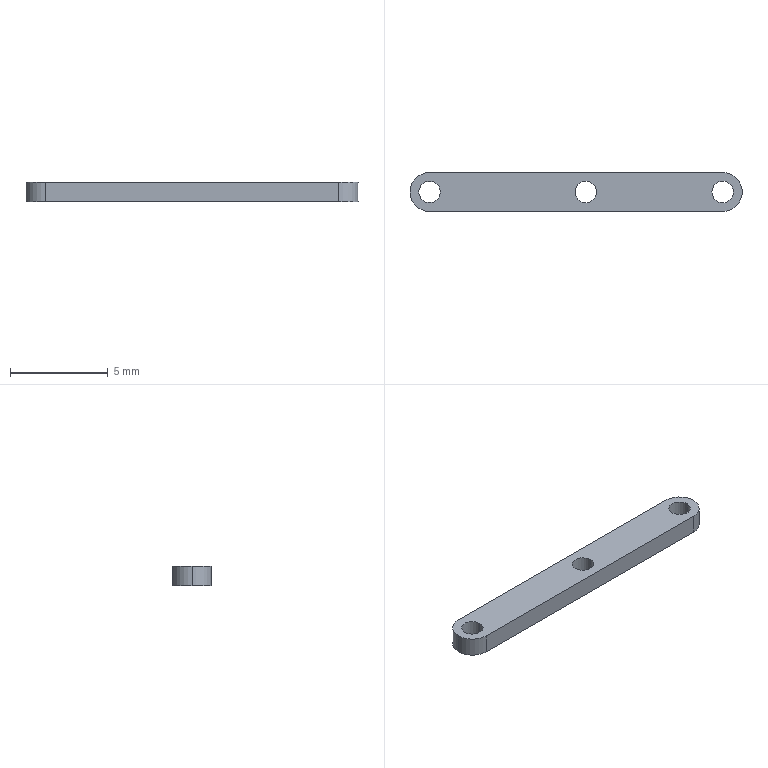Part | SolidWorks | features Extrusion 1, ICE 1 | 1 solid | 13 faces | box 17 x 2 x 1 mm | volume 30.291 mm3 | cylinder 9 | plane 4 | commonest cylinder face diameters 1.1 x6 2 x3
STEP:
#1=CARTESIAN_POINT('',(-0.05,0.,0.5));
#2=VERTEX_POINT('',#1);
#3=CARTESIAN_POINT('',(1.05,0.,0.5));
#4=VERTEX_POINT('',#3);
#5=CARTESIAN_POINT('',(0.5,0.,0.5));
#6=DIRECTION('',(0.,0.,1.));
#7=DIRECTION('',(1.,0.,0.));
#8=AXIS2_PLACEMENT_3D('',#5,#6,#7);
#9=CIRCLE('',#8,0.55);
#10=EDGE_CURVE('',#2,#4,#9,.T.);
#11=ORIENTED_EDGE('',*,*,#10,.T.);
#12=CARTESIAN_POINT('',(1.05,0.,-0.5));
#13=VERTEX_POINT('',#12);
#14=CARTESIAN_POINT('',(1.05,0.,0.5));
#15=DIRECTION('',(0.,0.,-1.));
#16=VECTOR('',#15,1000.);
#17=LINE('',#14,#16);
#18=EDGE_CURVE('',#4,#13,#17,.T.);
#19=ORIENTED_EDGE('',*,*,#18,.T.);
#20=CARTESIAN_POINT('',(-0.05,0.,-0.5));
#21=VERTEX_POINT('',#20);
#22=CARTESIAN_POINT('',(0.5,0.,-0.5));
#23=DIRECTION('',(0.,0.,1.));
#24=DIRECTION('',(1.,0.,0.));
#25=AXIS2_PLACEMENT_3D('',#22,#23,#24);
#26=CIRCLE('',#25,0.55);
#27=EDGE_CURVE('',#21,#13,#26,.T.);
#28=ORIENTED_EDGE('',*,*,#27,.F.);
#29=CARTESIAN_POINT('',(-0.05,0.,0.5));
#30=DIRECTION('',(0.,0.,-1.));
#31=VECTOR('',#30,1000.);
#32=LINE('',#29,#31);
#33=EDGE_CURVE('',#2,#21,#32,.T.);
#34=ORIENTED_EDGE('',*,*,#33,.F.);
#35=EDGE_LOOP('',(#11,#19,#28,#34));
#36=FACE_OUTER_BOUND('',#35,.T.);
#37=CARTESIAN_POINT('',(0.5,0.,0.5));
#38=DIRECTION('',(0.,0.,-1.));
#39=DIRECTION('',(-1.,0.,0.));
#40=AXIS2_PLACEMENT_3D('',#37,#38,#39);
#41=CYLINDRICAL_SURFACE('',#40,0.55);
#42=ADVANCED_FACE('',(#36),#41,.F.);
#43=CARTESIAN_POINT('',(6.95,0.,0.5));
#44=VERTEX_POINT('',#43);
#45=CARTESIAN_POINT('',(8.05,0.,0.5));
#46=VERTEX_POINT('',#45);
#47=CARTESIAN_POINT('',(7.5,0.,0.5));
#48=DIRECTION('',(0.,0.,1.));
#49=DIRECTION('',(1.,0.,0.));
#50=AXIS2_PLACEMENT_3D('',#47,#48,#49);
#51=CIRCLE('',#50,0.55);
#52=EDGE_CURVE('',#44,#46,#51,.T.);
#53=ORIENTED_EDGE('',*,*,#52,.T.);
#54=CARTESIAN_POINT('',(8.05,0.,-0.5));
#55=VERTEX_POINT('',#54);
#56=CARTESIAN_POINT('',(8.05,0.,0.5));
#57=DIRECTION('',(0.,0.,-1.));
#58=VECTOR('',#57,1000.);
#59=LINE('',#56,#58);
#60=EDGE_CURVE('',#46,#55,#59,.T.);
#61=ORIENTED_EDGE('',*,*,#60,.T.);
#62=CARTESIAN_POINT('',(6.95,0.,-0.5));
#63=VERTEX_POINT('',#62);
#64=CARTESIAN_POINT('',(7.5,0.,-0.5));
#65=DIRECTION('',(0.,0.,1.));
#66=DIRECTION('',(1.,0.,0.));
#67=AXIS2_PLACEMENT_3D('',#64,#65,#66);
#68=CIRCLE('',#67,0.55);
#69=EDGE_CURVE('',#63,#55,#68,.T.);
#70=ORIENTED_EDGE('',*,*,#69,.F.);
#71=CARTESIAN_POINT('',(6.95,0.,0.5));
#72=DIRECTION('',(0.,0.,-1.));
#73=VECTOR('',#72,1000.);
#74=LINE('',#71,#73);
#75=EDGE_CURVE('',#44,#63,#74,.T.);
#76=ORIENTED_EDGE('',*,*,#75,.F.);
#77=EDGE_LOOP('',(#53,#61,#70,#76));
#78=FACE_OUTER_BOUND('',#77,.T.);
#79=CARTESIAN_POINT('',(7.5,0.,0.5));
#80=DIRECTION('',(0.,0.,-1.));
#81=DIRECTION('',(-1.,0.,0.));
#82=AXIS2_PLACEMENT_3D('',#79,#80,#81);
#83=CYLINDRICAL_SURFACE('',#82,0.55);
#84=ADVANCED_FACE('',(#78),#83,.F.);
#85=CARTESIAN_POINT('',(-8.05,0.,0.5));
#86=VERTEX_POINT('',#85);
#87=CARTESIAN_POINT('',(-6.95,0.,0.5));
#88=VERTEX_POINT('',#87);
#89=CARTESIAN_POINT('',(-7.5,0.,0.5));
#90=DIRECTION('',(0.,0.,1.));
#91=DIRECTION('',(1.,0.,0.));
#92=AXIS2_PLACEMENT_3D('',#89,#90,#91);
#93=CIRCLE('',#92,0.55);
#94=EDGE_CURVE('',#86,#88,#93,.T.);
#95=ORIENTED_EDGE('',*,*,#94,.T.);
#96=CARTESIAN_POINT('',(-6.95,0.,-0.5));
#97=VERTEX_POINT('',#96);
#98=CARTESIAN_POINT('',(-6.95,0.,0.5));
#99=DIRECTION('',(0.,0.,-1.));
#100=VECTOR('',#99,1000.);
#101=LINE('',#98,#100);
#102=EDGE_CURVE('',#88,#97,#101,.T.);
#103=ORIENTED_EDGE('',*,*,#102,.T.);
#104=CARTESIAN_POINT('',(-8.05,0.,-0.5));
#105=VERTEX_POINT('',#104);
#106=CARTESIAN_POINT('',(-7.5,0.,-0.5));
#107=DIRECTION('',(0.,0.,1.));
#108=DIRECTION('',(1.,0.,0.));
#109=AXIS2_PLACEMENT_3D('',#106,#107,#108);
#110=CIRCLE('',#109,0.55);
#111=EDGE_CURVE('',#105,#97,#110,.T.);
#112=ORIENTED_EDGE('',*,*,#111,.F.);
#113=CARTESIAN_POINT('',(-8.05,0.,0.5));
#114=DIRECTION('',(0.,0.,-1.));
#115=VECTOR('',#114,1000.);
#116=LINE('',#113,#115);
#117=EDGE_CURVE('',#86,#105,#116,.T.);
#118=ORIENTED_EDGE('',*,*,#117,.F.);
#119=EDGE_LOOP('',(#95,#103,#112,#118));
#120=FACE_OUTER_BOUND('',#119,.T.);
#121=CARTESIAN_POINT('',(-7.5,0.,0.5));
#122=DIRECTION('',(0.,0.,-1.));
#123=DIRECTION('',(-1.,0.,0.));
#124=AXIS2_PLACEMENT_3D('',#121,#122,#123);
#125=CYLINDRICAL_SURFACE('',#124,0.55);
#126=ADVANCED_FACE('',(#120),#125,.F.);
#127=CARTESIAN_POINT('',(-8.5,0.,0.5));
#128=VERTEX_POINT('',#127);
#129=CARTESIAN_POINT('',(-7.5,-1.,0.5));
#130=VERTEX_POINT('',#129);
#131=CARTESIAN_POINT('',(-7.5,0.,0.5));
#132=DIRECTION('',(0.,0.,1.));
#133=DIRECTION('',(1.,0.,0.));
#134=AXIS2_PLACEMENT_3D('',#131,#132,#133);
#135=CIRCLE('',#134,1.);
#136=EDGE_CURVE('',#128,#130,#135,.T.);
#137=ORIENTED_EDGE('',*,*,#136,.F.);
#138=CARTESIAN_POINT('',(-8.5,0.,-0.5));
#139=VERTEX_POINT('',#138);
#140=CARTESIAN_POINT('',(-8.5,0.,0.5));
#141=DIRECTION('',(0.,0.,-1.));
#142=VECTOR('',#141,1000.);
#143=LINE('',#140,#142);
#144=EDGE_CURVE('',#128,#139,#143,.T.);
#145=ORIENTED_EDGE('',*,*,#144,.T.);
#146=CARTESIAN_POINT('',(-7.5,-1.,-0.5));
#147=VERTEX_POINT('',#146);
#148=CARTESIAN_POINT('',(-7.5,0.,-0.5));
#149=DIRECTION('',(0.,0.,1.));
#150=DIRECTION('',(1.,0.,0.));
#151=AXIS2_PLACEMENT_3D('',#148,#149,#150);
#152=CIRCLE('',#151,1.);
#153=EDGE_CURVE('',#139,#147,#152,.T.);
#154=ORIENTED_EDGE('',*,*,#153,.T.);
#155=CARTESIAN_POINT('',(-7.5,-1.,0.5));
#156=DIRECTION('',(0.,0.,-1.));
#157=VECTOR('',#156,1000.);
#158=LINE('',#155,#157);
#159=EDGE_CURVE('',#130,#147,#158,.T.);
#160=ORIENTED_EDGE('',*,*,#159,.F.);
#161=EDGE_LOOP('',(#137,#145,#154,#160));
#162=FACE_OUTER_BOUND('',#161,.T.);
#163=CARTESIAN_POINT('',(-7.5,0.,0.5));
#164=DIRECTION('',(0.,0.,-1.));
#165=DIRECTION('',(-1.,0.,0.));
#166=AXIS2_PLACEMENT_3D('',#163,#164,#165);
#167=CYLINDRICAL_SURFACE('',#166,1.);
#168=ADVANCED_FACE('',(#162),#167,.T.);
#169=ORIENTED_EDGE('',*,*,#52,.F.);
#170=CARTESIAN_POINT('',(7.5,0.,0.5));
#171=DIRECTION('',(0.,0.,1.));
#172=DIRECTION('',(1.,0.,0.));
#173=AXIS2_PLACEMENT_3D('',#170,#171,#172);
#174=CIRCLE('',#173,0.55);
#175=EDGE_CURVE('',#46,#44,#174,.T.);
#176=ORIENTED_EDGE('',*,*,#175,.F.);
#177=EDGE_LOOP('',(#169,#176));
#178=FACE_BOUND('',#177,.T.);
#179=CARTESIAN_POINT('',(-7.5,1.,0.5));
#180=VERTEX_POINT('',#179);
#181=CARTESIAN_POINT('',(-7.5,0.,0.5));
#182=DIRECTION('',(0.,0.,1.));
#183=DIRECTION('',(1.,0.,0.));
#184=AXIS2_PLACEMENT_3D('',#181,#182,#183);
#185=CIRCLE('',#184,1.);
#186=EDGE_CURVE('',#180,#128,#185,.T.);
#187=ORIENTED_EDGE('',*,*,#186,.T.);
#188=ORIENTED_EDGE('',*,*,#136,.T.);
#189=CARTESIAN_POINT('',(7.5,-1.,0.5));
#190=VERTEX_POINT('',#189);
#191=CARTESIAN_POINT('',(-7.5,-1.,0.5));
#192=DIRECTION('',(1.,0.,0.));
#193=VECTOR('',#192,1000.);
#194=LINE('',#191,#193);
#195=EDGE_CURVE('',#130,#190,#194,.T.);
#196=ORIENTED_EDGE('',*,*,#195,.T.);
#197=CARTESIAN_POINT('',(7.5,1.,0.5));
#198=VERTEX_POINT('',#197);
#199=CARTESIAN_POINT('',(7.5,0.,0.5));
#200=DIRECTION('',(0.,0.,1.));
#201=DIRECTION('',(1.,0.,0.));
#202=AXIS2_PLACEMENT_3D('',#199,#200,#201);
#203=CIRCLE('',#202,1.);
#204=EDGE_CURVE('',#190,#198,#203,.T.);
#205=ORIENTED_EDGE('',*,*,#204,.T.);
#206=CARTESIAN_POINT('',(-7.5,1.,0.5));
#207=DIRECTION('',(-1.,0.,0.));
#208=VECTOR('',#207,1000.);
#209=LINE('',#206,#208);
#210=EDGE_CURVE('',#198,#180,#209,.T.);
#211=ORIENTED_EDGE('',*,*,#210,.T.);
#212=EDGE_LOOP('',(#187,#188,#196,#205,#211));
#213=FACE_OUTER_BOUND('',#212,.T.);
#214=ORIENTED_EDGE('',*,*,#94,.F.);
#215=CARTESIAN_POINT('',(-7.5,0.,0.5));
#216=DIRECTION('',(0.,0.,1.));
#217=DIRECTION('',(1.,0.,0.));
#218=AXIS2_PLACEMENT_3D('',#215,#216,#217);
#219=CIRCLE('',#218,0.55);
#220=EDGE_CURVE('',#88,#86,#219,.T.);
#221=ORIENTED_EDGE('',*,*,#220,.F.);
#222=EDGE_LOOP('',(#214,#221));
#223=FACE_BOUND('',#222,.T.);
#224=ORIENTED_EDGE('',*,*,#10,.F.);
#225=CARTESIAN_POINT('',(0.5,0.,0.5));
#226=DIRECTION('',(0.,0.,1.));
#227=DIRECTION('',(1.,0.,0.));
#228=AXIS2_PLACEMENT_3D('',#225,#226,#227);
#229=CIRCLE('',#228,0.55);
#230=EDGE_CURVE('',#4,#2,#229,.T.);
#231=ORIENTED_EDGE('',*,*,#230,.F.);
#232=EDGE_LOOP('',(#224,#231));
#233=FACE_BOUND('',#232,.T.);
#234=CARTESIAN_POINT('',(-7.5,0.,0.5));
#235=DIRECTION('',(0.,0.,1.));
#236=DIRECTION('',(1.,0.,0.));
#237=AXIS2_PLACEMENT_3D('',#234,#235,#236);
#238=PLANE('',#237);
#239=ADVANCED_FACE('',(#178,#213,#223,#233),#238,.T.);
#240=CARTESIAN_POINT('',(-7.5,1.,-0.5));
#241=VERTEX_POINT('',#240);
#242=CARTESIAN_POINT('',(-7.5,0.,-0.5));
#243=DIRECTION('',(0.,0.,1.));
#244=DIRECTION('',(1.,0.,0.));
#245=AXIS2_PLACEMENT_3D('',#242,#243,#244);
#246=CIRCLE('',#245,1.);
#247=EDGE_CURVE('',#241,#139,#246,.T.);
#248=ORIENTED_EDGE('',*,*,#247,.F.);
#249=CARTESIAN_POINT('',(7.5,1.,-0.5));
#250=VERTEX_POINT('',#249);
#251=CARTESIAN_POINT('',(-7.5,1.,-0.5));
#252=DIRECTION('',(-1.,0.,0.));
#253=VECTOR('',#252,1000.);
#254=LINE('',#251,#253);
#255=EDGE_CURVE('',#250,#241,#254,.T.);
#256=ORIENTED_EDGE('',*,*,#255,.F.);
#257=CARTESIAN_POINT('',(7.5,-1.,-0.5));
#258=VERTEX_POINT('',#257);
#259=CARTESIAN_POINT('',(7.5,0.,-0.5));
#260=DIRECTION('',(0.,0.,1.));
#261=DIRECTION('',(1.,0.,0.));
#262=AXIS2_PLACEMENT_3D('',#259,#260,#261);
#263=CIRCLE('',#262,1.);
#264=EDGE_CURVE('',#258,#250,#263,.T.);
#265=ORIENTED_EDGE('',*,*,#264,.F.);
#266=CARTESIAN_POINT('',(-7.5,-1.,-0.5));
#267=DIRECTION('',(1.,0.,0.));
#268=VECTOR('',#267,1000.);
#269=LINE('',#266,#268);
#270=EDGE_CURVE('',#147,#258,#269,.T.);
#271=ORIENTED_EDGE('',*,*,#270,.F.);
#272=ORIENTED_EDGE('',*,*,#153,.F.);
#273=EDGE_LOOP('',(#248,#256,#265,#271,#272));
#274=FACE_OUTER_BOUND('',#273,.T.);
#275=ORIENTED_EDGE('',*,*,#111,.T.);
#276=CARTESIAN_POINT('',(-7.5,0.,-0.5));
#277=DIRECTION('',(0.,0.,1.));
#278=DIRECTION('',(1.,0.,0.));
#279=AXIS2_PLACEMENT_3D('',#276,#277,#278);
#280=CIRCLE('',#279,0.55);
#281=EDGE_CURVE('',#97,#105,#280,.T.);
#282=ORIENTED_EDGE('',*,*,#281,.T.);
#283=EDGE_LOOP('',(#275,#282));
#284=FACE_BOUND('',#283,.T.);
#285=ORIENTED_EDGE('',*,*,#69,.T.);
#286=CARTESIAN_POINT('',(7.5,0.,-0.5));
#287=DIRECTION('',(0.,0.,1.));
#288=DIRECTION('',(1.,0.,0.));
#289=AXIS2_PLACEMENT_3D('',#286,#287,#288);
#290=CIRCLE('',#289,0.55);
#291=EDGE_CURVE('',#55,#63,#290,.T.);
#292=ORIENTED_EDGE('',*,*,#291,.T.);
#293=EDGE_LOOP('',(#285,#292));
#294=FACE_BOUND('',#293,.T.);
#295=ORIENTED_EDGE('',*,*,#27,.T.);
#296=CARTESIAN_POINT('',(0.5,0.,-0.5));
#297=DIRECTION('',(0.,0.,1.));
#298=DIRECTION('',(1.,0.,0.));
#299=AXIS2_PLACEMENT_3D('',#296,#297,#298);
#300=CIRCLE('',#299,0.55);
#301=EDGE_CURVE('',#13,#21,#300,.T.);
#302=ORIENTED_EDGE('',*,*,#301,.T.);
#303=EDGE_LOOP('',(#295,#302));
#304=FACE_BOUND('',#303,.T.);
#305=CARTESIAN_POINT('',(-7.5,0.,-0.5));
#306=DIRECTION('',(0.,0.,1.));
#307=DIRECTION('',(1.,0.,0.));
#308=AXIS2_PLACEMENT_3D('',#305,#306,#307);
#309=PLANE('',#308);
#310=ADVANCED_FACE('',(#274,#284,#294,#304),#309,.F.);
#311=ORIENTED_EDGE('',*,*,#144,.F.);
#312=ORIENTED_EDGE('',*,*,#186,.F.);
#313=CARTESIAN_POINT('',(-7.5,1.,0.5));
#314=DIRECTION('',(0.,0.,-1.));
#315=VECTOR('',#314,1000.);
#316=LINE('',#313,#315);
#317=EDGE_CURVE('',#180,#241,#316,.T.);
#318=ORIENTED_EDGE('',*,*,#317,.T.);
#319=ORIENTED_EDGE('',*,*,#247,.T.);
#320=EDGE_LOOP('',(#311,#312,#318,#319));
#321=FACE_OUTER_BOUND('',#320,.T.);
#322=CARTESIAN_POINT('',(-7.5,0.,0.5));
#323=DIRECTION('',(0.,0.,-1.));
#324=DIRECTION('',(-1.,0.,0.));
#325=AXIS2_PLACEMENT_3D('',#322,#323,#324);
#326=CYLINDRICAL_SURFACE('',#325,1.);
#327=ADVANCED_FACE('',(#321),#326,.T.);
#328=ORIENTED_EDGE('',*,*,#270,.T.);
#329=CARTESIAN_POINT('',(7.5,-1.,0.5));
#330=DIRECTION('',(0.,0.,-1.));
#331=VECTOR('',#330,1000.);
#332=LINE('',#329,#331);
#333=EDGE_CURVE('',#190,#258,#332,.T.);
#334=ORIENTED_EDGE('',*,*,#333,.F.);
#335=ORIENTED_EDGE('',*,*,#195,.F.);
#336=ORIENTED_EDGE('',*,*,#159,.T.);
#337=EDGE_LOOP('',(#328,#334,#335,#336));
#338=FACE_OUTER_BOUND('',#337,.T.);
#339=CARTESIAN_POINT('',(-7.5,-1.,0.5));
#340=DIRECTION('',(0.,1.,0.));
#341=DIRECTION('',(-1.,0.,0.));
#342=AXIS2_PLACEMENT_3D('',#339,#340,#341);
#343=PLANE('',#342);
#344=ADVANCED_FACE('',(#338),#343,.F.);
#345=ORIENTED_EDGE('',*,*,#264,.T.);
#346=CARTESIAN_POINT('',(7.5,1.,0.5));
#347=DIRECTION('',(0.,0.,-1.));
#348=VECTOR('',#347,1000.);
#349=LINE('',#346,#348);
#350=EDGE_CURVE('',#198,#250,#349,.T.);
#351=ORIENTED_EDGE('',*,*,#350,.F.);
#352=ORIENTED_EDGE('',*,*,#204,.F.);
#353=ORIENTED_EDGE('',*,*,#333,.T.);
#354=EDGE_LOOP('',(#345,#351,#352,#353));
#355=FACE_OUTER_BOUND('',#354,.T.);
#356=CARTESIAN_POINT('',(7.5,0.,0.5));
#357=DIRECTION('',(0.,0.,-1.));
#358=DIRECTION('',(-1.,0.,0.));
#359=AXIS2_PLACEMENT_3D('',#356,#357,#358);
#360=CYLINDRICAL_SURFACE('',#359,1.);
#361=ADVANCED_FACE('',(#355),#360,.T.);
#362=ORIENTED_EDGE('',*,*,#255,.T.);
#363=ORIENTED_EDGE('',*,*,#317,.F.);
#364=ORIENTED_EDGE('',*,*,#210,.F.);
#365=ORIENTED_EDGE('',*,*,#350,.T.);
#366=EDGE_LOOP('',(#362,#363,#364,#365));
#367=FACE_OUTER_BOUND('',#366,.T.);
#368=CARTESIAN_POINT('',(-7.5,1.,0.5));
#369=DIRECTION('',(0.,-1.,0.));
#370=DIRECTION('',(1.,0.,0.));
#371=AXIS2_PLACEMENT_3D('',#368,#369,#370);
#372=PLANE('',#371);
#373=ADVANCED_FACE('',(#367),#372,.F.);
#374=ORIENTED_EDGE('',*,*,#102,.F.);
#375=ORIENTED_EDGE('',*,*,#220,.T.);
#376=ORIENTED_EDGE('',*,*,#117,.T.);
#377=ORIENTED_EDGE('',*,*,#281,.F.);
#378=EDGE_LOOP('',(#374,#375,#376,#377));
#379=FACE_OUTER_BOUND('',#378,.T.);
#380=CARTESIAN_POINT('',(-7.5,0.,0.5));
#381=DIRECTION('',(0.,0.,-1.));
#382=DIRECTION('',(-1.,0.,0.));
#383=AXIS2_PLACEMENT_3D('',#380,#381,#382);
#384=CYLINDRICAL_SURFACE('',#383,0.55);
#385=ADVANCED_FACE('',(#379),#384,.F.);
#386=ORIENTED_EDGE('',*,*,#60,.F.);
#387=ORIENTED_EDGE('',*,*,#175,.T.);
#388=ORIENTED_EDGE('',*,*,#75,.T.);
#389=ORIENTED_EDGE('',*,*,#291,.F.);
#390=EDGE_LOOP('',(#386,#387,#388,#389));
#391=FACE_OUTER_BOUND('',#390,.T.);
#392=CARTESIAN_POINT('',(7.5,0.,0.5));
#393=DIRECTION('',(0.,0.,-1.));
#394=DIRECTION('',(-1.,0.,0.));
#395=AXIS2_PLACEMENT_3D('',#392,#393,#394);
#396=CYLINDRICAL_SURFACE('',#395,0.55);
#397=ADVANCED_FACE('',(#391),#396,.F.);
#398=ORIENTED_EDGE('',*,*,#18,.F.);
#399=ORIENTED_EDGE('',*,*,#230,.T.);
#400=ORIENTED_EDGE('',*,*,#33,.T.);
#401=ORIENTED_EDGE('',*,*,#301,.F.);
#402=EDGE_LOOP('',(#398,#399,#400,#401));
#403=FACE_OUTER_BOUND('',#402,.T.);
#404=CARTESIAN_POINT('',(0.5,0.,0.5));
#405=DIRECTION('',(0.,0.,-1.));
#406=DIRECTION('',(-1.,0.,0.));
#407=AXIS2_PLACEMENT_3D('',#404,#405,#406);
#408=CYLINDRICAL_SURFACE('',#407,0.55);
#409=ADVANCED_FACE('',(#403),#408,.F.);
#410=CLOSED_SHELL('',(#42,#84,#126,#168,#239,#310,#327,#344,#361,#373,#385,#397,#409));
#411=MANIFOLD_SOLID_BREP('',#410);
#412=CARTESIAN_POINT('',(0.,0.,0.));
#413=DIRECTION('',(0.,0.,1.));
#414=DIRECTION('',(1.,0.,0.));
#415=AXIS2_PLACEMENT_3D('',#412,#413,#414);
#416=(LENGTH_UNIT()NAMED_UNIT(*)SI_UNIT(.MILLI.,.METRE.));
#417=UNCERTAINTY_MEASURE_WITH_UNIT(LENGTH_MEASURE(0.00001),#416,'','');
#418=(NAMED_UNIT(*)PLANE_ANGLE_UNIT()SI_UNIT($,.RADIAN.));
#419=(NAMED_UNIT(*)SI_UNIT($,.STERADIAN.)SOLID_ANGLE_UNIT());
#420=(GEOMETRIC_REPRESENTATION_CONTEXT(3)GLOBAL_UNCERTAINTY_ASSIGNED_CONTEXT((#417))GLOBAL_UNIT_ASSIGNED_CONTEXT((#416,#418,#419))REPRESENTATION_CONTEXT('',''));
#421=ADVANCED_BREP_SHAPE_REPRESENTATION('',(#411,#415),#420);